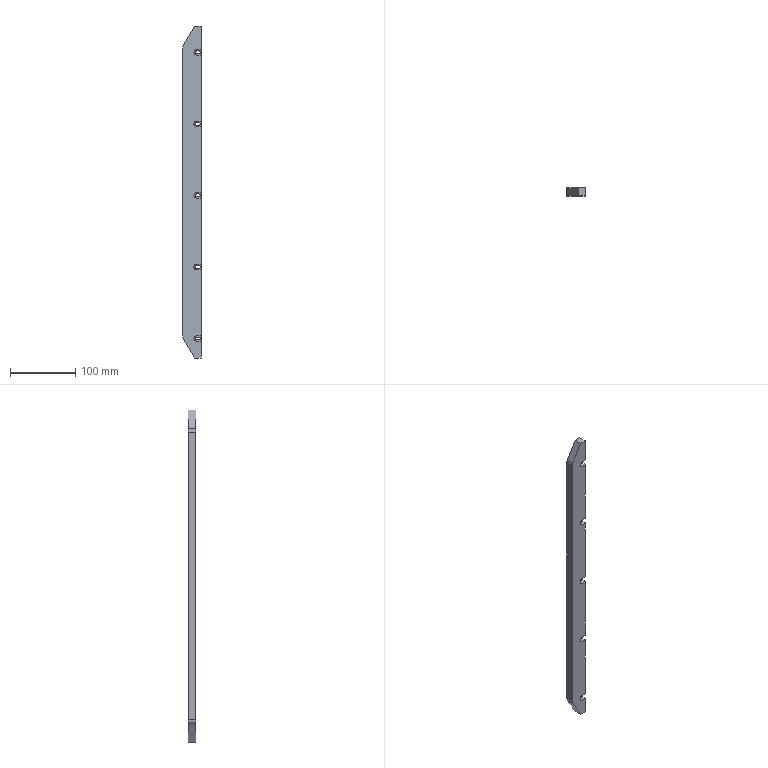Part | STEP file | Tdangtiao-001_デフォルト | 1 solid | 50 faces | box 28 x 12 x 510.5 mm | volume 161527 mm3 | plane 33 | cylinder 17 | commonest cylinder face diameters 4.5 x10 8.5 x5 20 x2